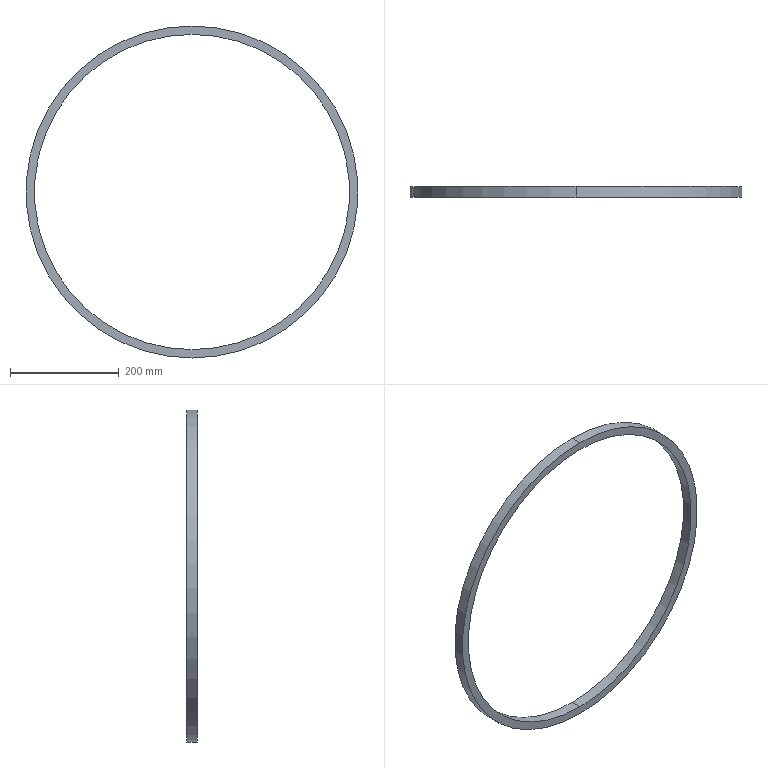Part | SolidWorks | features Extrusion 1 | 1 solid | 6 faces | box 610 x 20 x 610 mm | volume 578980 mm3 | cylinder 4 | plane 2 | commonest cylinder face diameters 579 x2 610 x2
STEP:
#1=CARTESIAN_POINT('',(0.,20.,-289.5));
#2=VERTEX_POINT('',#1);
#3=CARTESIAN_POINT('',(0.,20.,289.5));
#4=VERTEX_POINT('',#3);
#5=CARTESIAN_POINT('',(0.,20.,0.));
#6=DIRECTION('',(0.,1.,0.));
#7=DIRECTION('',(0.,0.,1.));
#8=AXIS2_PLACEMENT_3D('',#5,#6,#7);
#9=CIRCLE('',#8,289.5);
#10=EDGE_CURVE('',#2,#4,#9,.T.);
#11=ORIENTED_EDGE('',*,*,#10,.T.);
#12=CARTESIAN_POINT('',(0.,0.,289.5));
#13=VERTEX_POINT('',#12);
#14=CARTESIAN_POINT('',(0.,20.,289.5));
#15=DIRECTION('',(0.,-1.,0.));
#16=VECTOR('',#15,1000.);
#17=LINE('',#14,#16);
#18=EDGE_CURVE('',#4,#13,#17,.T.);
#19=ORIENTED_EDGE('',*,*,#18,.T.);
#20=CARTESIAN_POINT('',(0.,0.,-289.5));
#21=VERTEX_POINT('',#20);
#22=CARTESIAN_POINT('',(0.,0.,0.));
#23=DIRECTION('',(0.,1.,0.));
#24=DIRECTION('',(0.,0.,1.));
#25=AXIS2_PLACEMENT_3D('',#22,#23,#24);
#26=CIRCLE('',#25,289.5);
#27=EDGE_CURVE('',#21,#13,#26,.T.);
#28=ORIENTED_EDGE('',*,*,#27,.F.);
#29=CARTESIAN_POINT('',(0.,20.,-289.5));
#30=DIRECTION('',(0.,-1.,0.));
#31=VECTOR('',#30,1000.);
#32=LINE('',#29,#31);
#33=EDGE_CURVE('',#2,#21,#32,.T.);
#34=ORIENTED_EDGE('',*,*,#33,.F.);
#35=EDGE_LOOP('',(#11,#19,#28,#34));
#36=FACE_OUTER_BOUND('',#35,.T.);
#37=CARTESIAN_POINT('',(0.,20.,0.));
#38=DIRECTION('',(0.,-1.,0.));
#39=DIRECTION('',(0.,0.,-1.));
#40=AXIS2_PLACEMENT_3D('',#37,#38,#39);
#41=CYLINDRICAL_SURFACE('',#40,289.5);
#42=ADVANCED_FACE('',(#36),#41,.F.);
#43=CARTESIAN_POINT('',(0.,20.,305.));
#44=VERTEX_POINT('',#43);
#45=CARTESIAN_POINT('',(0.,20.,-305.));
#46=VERTEX_POINT('',#45);
#47=CARTESIAN_POINT('',(0.,20.,0.));
#48=DIRECTION('',(0.,1.,0.));
#49=DIRECTION('',(0.,0.,1.));
#50=AXIS2_PLACEMENT_3D('',#47,#48,#49);
#51=CIRCLE('',#50,305.);
#52=EDGE_CURVE('',#44,#46,#51,.T.);
#53=ORIENTED_EDGE('',*,*,#52,.F.);
#54=CARTESIAN_POINT('',(0.,0.,305.));
#55=VERTEX_POINT('',#54);
#56=CARTESIAN_POINT('',(0.,20.,305.));
#57=DIRECTION('',(0.,-1.,0.));
#58=VECTOR('',#57,1000.);
#59=LINE('',#56,#58);
#60=EDGE_CURVE('',#44,#55,#59,.T.);
#61=ORIENTED_EDGE('',*,*,#60,.T.);
#62=CARTESIAN_POINT('',(0.,0.,-305.));
#63=VERTEX_POINT('',#62);
#64=CARTESIAN_POINT('',(0.,0.,0.));
#65=DIRECTION('',(0.,1.,0.));
#66=DIRECTION('',(0.,0.,1.));
#67=AXIS2_PLACEMENT_3D('',#64,#65,#66);
#68=CIRCLE('',#67,305.);
#69=EDGE_CURVE('',#55,#63,#68,.T.);
#70=ORIENTED_EDGE('',*,*,#69,.T.);
#71=CARTESIAN_POINT('',(0.,20.,-305.));
#72=DIRECTION('',(0.,-1.,0.));
#73=VECTOR('',#72,1000.);
#74=LINE('',#71,#73);
#75=EDGE_CURVE('',#46,#63,#74,.T.);
#76=ORIENTED_EDGE('',*,*,#75,.F.);
#77=EDGE_LOOP('',(#53,#61,#70,#76));
#78=FACE_OUTER_BOUND('',#77,.T.);
#79=CARTESIAN_POINT('',(0.,20.,0.));
#80=DIRECTION('',(0.,-1.,0.));
#81=DIRECTION('',(0.,0.,-1.));
#82=AXIS2_PLACEMENT_3D('',#79,#80,#81);
#83=CYLINDRICAL_SURFACE('',#82,305.);
#84=ADVANCED_FACE('',(#78),#83,.T.);
#85=CARTESIAN_POINT('',(0.,20.,0.));
#86=DIRECTION('',(0.,1.,0.));
#87=DIRECTION('',(0.,0.,1.));
#88=AXIS2_PLACEMENT_3D('',#85,#86,#87);
#89=CIRCLE('',#88,305.);
#90=EDGE_CURVE('',#46,#44,#89,.T.);
#91=ORIENTED_EDGE('',*,*,#90,.T.);
#92=ORIENTED_EDGE('',*,*,#52,.T.);
#93=EDGE_LOOP('',(#91,#92));
#94=FACE_OUTER_BOUND('',#93,.T.);
#95=ORIENTED_EDGE('',*,*,#10,.F.);
#96=CARTESIAN_POINT('',(0.,20.,0.));
#97=DIRECTION('',(0.,1.,0.));
#98=DIRECTION('',(0.,0.,1.));
#99=AXIS2_PLACEMENT_3D('',#96,#97,#98);
#100=CIRCLE('',#99,289.5);
#101=EDGE_CURVE('',#4,#2,#100,.T.);
#102=ORIENTED_EDGE('',*,*,#101,.F.);
#103=EDGE_LOOP('',(#95,#102));
#104=FACE_BOUND('',#103,.T.);
#105=CARTESIAN_POINT('',(0.,20.,0.));
#106=DIRECTION('',(0.,1.,0.));
#107=DIRECTION('',(0.,0.,1.));
#108=AXIS2_PLACEMENT_3D('',#105,#106,#107);
#109=PLANE('',#108);
#110=ADVANCED_FACE('',(#94,#104),#109,.T.);
#111=CARTESIAN_POINT('',(0.,0.,0.));
#112=DIRECTION('',(0.,1.,0.));
#113=DIRECTION('',(0.,0.,1.));
#114=AXIS2_PLACEMENT_3D('',#111,#112,#113);
#115=CIRCLE('',#114,305.);
#116=EDGE_CURVE('',#63,#55,#115,.T.);
#117=ORIENTED_EDGE('',*,*,#116,.F.);
#118=ORIENTED_EDGE('',*,*,#69,.F.);
#119=EDGE_LOOP('',(#117,#118));
#120=FACE_OUTER_BOUND('',#119,.T.);
#121=ORIENTED_EDGE('',*,*,#27,.T.);
#122=CARTESIAN_POINT('',(0.,0.,0.));
#123=DIRECTION('',(0.,1.,0.));
#124=DIRECTION('',(0.,0.,1.));
#125=AXIS2_PLACEMENT_3D('',#122,#123,#124);
#126=CIRCLE('',#125,289.5);
#127=EDGE_CURVE('',#13,#21,#126,.T.);
#128=ORIENTED_EDGE('',*,*,#127,.T.);
#129=EDGE_LOOP('',(#121,#128));
#130=FACE_BOUND('',#129,.T.);
#131=CARTESIAN_POINT('',(0.,0.,0.));
#132=DIRECTION('',(0.,1.,0.));
#133=DIRECTION('',(0.,0.,1.));
#134=AXIS2_PLACEMENT_3D('',#131,#132,#133);
#135=PLANE('',#134);
#136=ADVANCED_FACE('',(#120,#130),#135,.F.);
#137=ORIENTED_EDGE('',*,*,#60,.F.);
#138=ORIENTED_EDGE('',*,*,#90,.F.);
#139=ORIENTED_EDGE('',*,*,#75,.T.);
#140=ORIENTED_EDGE('',*,*,#116,.T.);
#141=EDGE_LOOP('',(#137,#138,#139,#140));
#142=FACE_OUTER_BOUND('',#141,.T.);
#143=CARTESIAN_POINT('',(0.,20.,0.));
#144=DIRECTION('',(0.,-1.,0.));
#145=DIRECTION('',(0.,0.,-1.));
#146=AXIS2_PLACEMENT_3D('',#143,#144,#145);
#147=CYLINDRICAL_SURFACE('',#146,305.);
#148=ADVANCED_FACE('',(#142),#147,.T.);
#149=ORIENTED_EDGE('',*,*,#18,.F.);
#150=ORIENTED_EDGE('',*,*,#101,.T.);
#151=ORIENTED_EDGE('',*,*,#33,.T.);
#152=ORIENTED_EDGE('',*,*,#127,.F.);
#153=EDGE_LOOP('',(#149,#150,#151,#152));
#154=FACE_OUTER_BOUND('',#153,.T.);
#155=CARTESIAN_POINT('',(0.,20.,0.));
#156=DIRECTION('',(0.,-1.,0.));
#157=DIRECTION('',(0.,0.,-1.));
#158=AXIS2_PLACEMENT_3D('',#155,#156,#157);
#159=CYLINDRICAL_SURFACE('',#158,289.5);
#160=ADVANCED_FACE('',(#154),#159,.F.);
#161=CLOSED_SHELL('',(#42,#84,#110,#136,#148,#160));
#162=MANIFOLD_SOLID_BREP('',#161);
#163=CARTESIAN_POINT('',(0.,0.,0.));
#164=DIRECTION('',(0.,0.,1.));
#165=DIRECTION('',(1.,0.,0.));
#166=AXIS2_PLACEMENT_3D('',#163,#164,#165);
#167=(LENGTH_UNIT()NAMED_UNIT(*)SI_UNIT(.MILLI.,.METRE.));
#168=UNCERTAINTY_MEASURE_WITH_UNIT(LENGTH_MEASURE(0.00001),#167,'','');
#169=(NAMED_UNIT(*)PLANE_ANGLE_UNIT()SI_UNIT($,.RADIAN.));
#170=(NAMED_UNIT(*)SI_UNIT($,.STERADIAN.)SOLID_ANGLE_UNIT());
#171=(GEOMETRIC_REPRESENTATION_CONTEXT(3)GLOBAL_UNCERTAINTY_ASSIGNED_CONTEXT((#168))GLOBAL_UNIT_ASSIGNED_CONTEXT((#167,#169,#170))REPRESENTATION_CONTEXT('',''));
#172=ADVANCED_BREP_SHAPE_REPRESENTATION('',(#162,#166),#171);